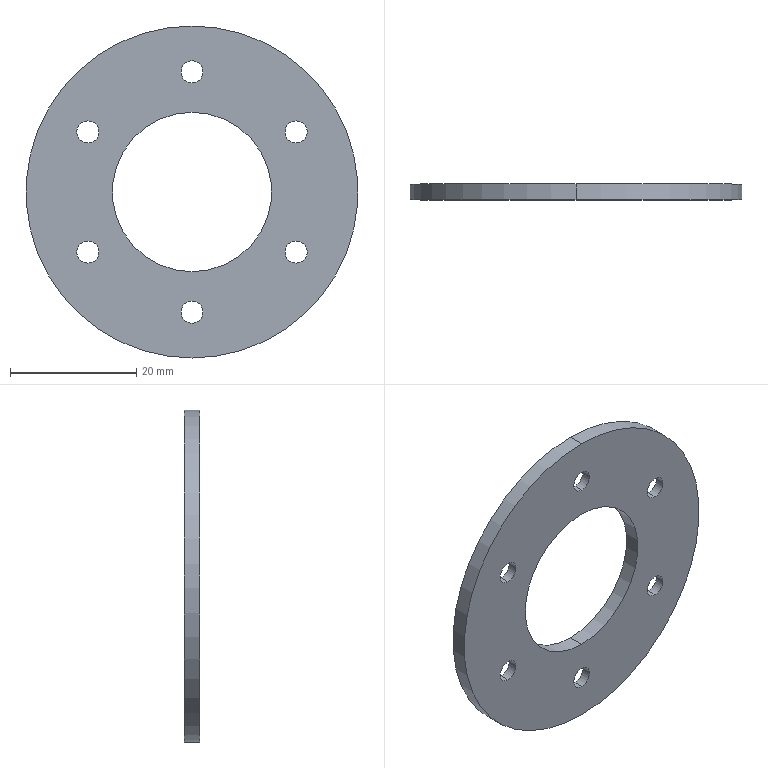Part | SolidWorks | features ICE 4, CirPattern 2, Chamfer 1, Extrusion 1 | 1 solid | 36 faces | box 52.5 x 2.5 x 52.5 mm | volume 3777 mm3 | cylinder 28 | plane 8 | commonest cylinder face diameters 3.5 x12 8 x12 25.2 x2 52.5 x2
STEP:
#1=CARTESIAN_POINT('',(-16.454,1.5,-13.5));
#2=VERTEX_POINT('',#1);
#3=CARTESIAN_POINT('',(-16.454,1.5,-5.5));
#4=VERTEX_POINT('',#3);
#5=CARTESIAN_POINT('',(-16.454,1.5,-9.5));
#6=DIRECTION('',(0.,1.,0.));
#7=DIRECTION('',(0.866,0.,0.5));
#8=AXIS2_PLACEMENT_3D('',#5,#6,#7);
#9=CIRCLE('',#8,4.);
#10=EDGE_CURVE('',#2,#4,#9,.T.);
#11=ORIENTED_EDGE('',*,*,#10,.F.);
#12=CARTESIAN_POINT('',(-16.454,2.5,-13.5));
#13=VERTEX_POINT('',#12);
#14=CARTESIAN_POINT('',(-16.454,1.5,-13.5));
#15=DIRECTION('',(0.,1.,0.));
#16=VECTOR('',#15,1000.);
#17=LINE('',#14,#16);
#18=EDGE_CURVE('',#2,#13,#17,.T.);
#19=ORIENTED_EDGE('',*,*,#18,.T.);
#20=CARTESIAN_POINT('',(-16.454,2.5,-5.5));
#21=VERTEX_POINT('',#20);
#22=CARTESIAN_POINT('',(-16.454,2.5,-9.5));
#23=DIRECTION('',(0.,1.,0.));
#24=DIRECTION('',(0.866,0.,0.5));
#25=AXIS2_PLACEMENT_3D('',#22,#23,#24);
#26=CIRCLE('',#25,4.);
#27=EDGE_CURVE('',#13,#21,#26,.T.);
#28=ORIENTED_EDGE('',*,*,#27,.T.);
#29=CARTESIAN_POINT('',(-16.454,1.5,-5.5));
#30=DIRECTION('',(0.,1.,0.));
#31=VECTOR('',#30,1000.);
#32=LINE('',#29,#31);
#33=EDGE_CURVE('',#4,#21,#32,.T.);
#34=ORIENTED_EDGE('',*,*,#33,.F.);
#35=EDGE_LOOP('',(#11,#19,#28,#34));
#36=FACE_OUTER_BOUND('',#35,.T.);
#37=CARTESIAN_POINT('',(-16.454,1.5,-9.5));
#38=DIRECTION('',(0.,1.,0.));
#39=DIRECTION('',(0.,0.,1.));
#40=AXIS2_PLACEMENT_3D('',#37,#38,#39);
#41=CYLINDRICAL_SURFACE('',#40,4.);
#42=ADVANCED_FACE('',(#36),#41,.F.);
#43=CARTESIAN_POINT('',(-16.454,1.5,5.5));
#44=VERTEX_POINT('',#43);
#45=CARTESIAN_POINT('',(-16.454,1.5,13.5));
#46=VERTEX_POINT('',#45);
#47=CARTESIAN_POINT('',(-16.454,1.5,9.5));
#48=DIRECTION('',(0.,1.,0.));
#49=DIRECTION('',(0.866,0.,-0.5));
#50=AXIS2_PLACEMENT_3D('',#47,#48,#49);
#51=CIRCLE('',#50,4.);
#52=EDGE_CURVE('',#44,#46,#51,.T.);
#53=ORIENTED_EDGE('',*,*,#52,.F.);
#54=CARTESIAN_POINT('',(-16.454,2.5,5.5));
#55=VERTEX_POINT('',#54);
#56=CARTESIAN_POINT('',(-16.454,1.5,5.5));
#57=DIRECTION('',(0.,1.,0.));
#58=VECTOR('',#57,1000.);
#59=LINE('',#56,#58);
#60=EDGE_CURVE('',#44,#55,#59,.T.);
#61=ORIENTED_EDGE('',*,*,#60,.T.);
#62=CARTESIAN_POINT('',(-16.454,2.5,13.5));
#63=VERTEX_POINT('',#62);
#64=CARTESIAN_POINT('',(-16.454,2.5,9.5));
#65=DIRECTION('',(0.,1.,0.));
#66=DIRECTION('',(0.866,0.,-0.5));
#67=AXIS2_PLACEMENT_3D('',#64,#65,#66);
#68=CIRCLE('',#67,4.);
#69=EDGE_CURVE('',#55,#63,#68,.T.);
#70=ORIENTED_EDGE('',*,*,#69,.T.);
#71=CARTESIAN_POINT('',(-16.454,1.5,13.5));
#72=DIRECTION('',(0.,1.,0.));
#73=VECTOR('',#72,1000.);
#74=LINE('',#71,#73);
#75=EDGE_CURVE('',#46,#63,#74,.T.);
#76=ORIENTED_EDGE('',*,*,#75,.F.);
#77=EDGE_LOOP('',(#53,#61,#70,#76));
#78=FACE_OUTER_BOUND('',#77,.T.);
#79=CARTESIAN_POINT('',(-16.454,1.5,9.5));
#80=DIRECTION('',(0.,1.,0.));
#81=DIRECTION('',(0.,0.,1.));
#82=AXIS2_PLACEMENT_3D('',#79,#80,#81);
#83=CYLINDRICAL_SURFACE('',#82,4.);
#84=ADVANCED_FACE('',(#78),#83,.F.);
#85=CARTESIAN_POINT('',(0.,1.5,15.));
#86=VERTEX_POINT('',#85);
#87=CARTESIAN_POINT('',(0.,1.5,23.));
#88=VERTEX_POINT('',#87);
#89=CARTESIAN_POINT('',(0.,1.5,19.));
#90=DIRECTION('',(0.,1.,0.));
#91=DIRECTION('',(0.,0.,-1.));
#92=AXIS2_PLACEMENT_3D('',#89,#90,#91);
#93=CIRCLE('',#92,4.);
#94=EDGE_CURVE('',#86,#88,#93,.T.);
#95=ORIENTED_EDGE('',*,*,#94,.F.);
#96=CARTESIAN_POINT('',(0.,2.5,15.));
#97=VERTEX_POINT('',#96);
#98=CARTESIAN_POINT('',(0.,1.5,15.));
#99=DIRECTION('',(0.,1.,0.));
#100=VECTOR('',#99,1000.);
#101=LINE('',#98,#100);
#102=EDGE_CURVE('',#86,#97,#101,.T.);
#103=ORIENTED_EDGE('',*,*,#102,.T.);
#104=CARTESIAN_POINT('',(0.,2.5,23.));
#105=VERTEX_POINT('',#104);
#106=CARTESIAN_POINT('',(0.,2.5,19.));
#107=DIRECTION('',(0.,1.,0.));
#108=DIRECTION('',(0.,0.,-1.));
#109=AXIS2_PLACEMENT_3D('',#106,#107,#108);
#110=CIRCLE('',#109,4.);
#111=EDGE_CURVE('',#97,#105,#110,.T.);
#112=ORIENTED_EDGE('',*,*,#111,.T.);
#113=CARTESIAN_POINT('',(0.,1.5,23.));
#114=DIRECTION('',(0.,1.,0.));
#115=VECTOR('',#114,1000.);
#116=LINE('',#113,#115);
#117=EDGE_CURVE('',#88,#105,#116,.T.);
#118=ORIENTED_EDGE('',*,*,#117,.F.);
#119=EDGE_LOOP('',(#95,#103,#112,#118));
#120=FACE_OUTER_BOUND('',#119,.T.);
#121=CARTESIAN_POINT('',(0.,1.5,19.));
#122=DIRECTION('',(0.,1.,0.));
#123=DIRECTION('',(0.,0.,1.));
#124=AXIS2_PLACEMENT_3D('',#121,#122,#123);
#125=CYLINDRICAL_SURFACE('',#124,4.);
#126=ADVANCED_FACE('',(#120),#125,.F.);
#127=CARTESIAN_POINT('',(16.454,1.5,5.5));
#128=VERTEX_POINT('',#127);
#129=CARTESIAN_POINT('',(16.454,1.5,13.5));
#130=VERTEX_POINT('',#129);
#131=CARTESIAN_POINT('',(16.454,1.5,9.5));
#132=DIRECTION('',(0.,1.,0.));
#133=DIRECTION('',(-0.866,0.,-0.5));
#134=AXIS2_PLACEMENT_3D('',#131,#132,#133);
#135=CIRCLE('',#134,4.);
#136=EDGE_CURVE('',#128,#130,#135,.T.);
#137=ORIENTED_EDGE('',*,*,#136,.F.);
#138=CARTESIAN_POINT('',(16.454,2.5,5.5));
#139=VERTEX_POINT('',#138);
#140=CARTESIAN_POINT('',(16.454,1.5,5.5));
#141=DIRECTION('',(0.,1.,0.));
#142=VECTOR('',#141,1000.);
#143=LINE('',#140,#142);
#144=EDGE_CURVE('',#128,#139,#143,.T.);
#145=ORIENTED_EDGE('',*,*,#144,.T.);
#146=CARTESIAN_POINT('',(16.454,2.5,13.5));
#147=VERTEX_POINT('',#146);
#148=CARTESIAN_POINT('',(16.454,2.5,9.5));
#149=DIRECTION('',(0.,1.,0.));
#150=DIRECTION('',(-0.866,0.,-0.5));
#151=AXIS2_PLACEMENT_3D('',#148,#149,#150);
#152=CIRCLE('',#151,4.);
#153=EDGE_CURVE('',#139,#147,#152,.T.);
#154=ORIENTED_EDGE('',*,*,#153,.T.);
#155=CARTESIAN_POINT('',(16.454,1.5,13.5));
#156=DIRECTION('',(0.,1.,0.));
#157=VECTOR('',#156,1000.);
#158=LINE('',#155,#157);
#159=EDGE_CURVE('',#130,#147,#158,.T.);
#160=ORIENTED_EDGE('',*,*,#159,.F.);
#161=EDGE_LOOP('',(#137,#145,#154,#160));
#162=FACE_OUTER_BOUND('',#161,.T.);
#163=CARTESIAN_POINT('',(16.454,1.5,9.5));
#164=DIRECTION('',(0.,1.,0.));
#165=DIRECTION('',(0.,0.,1.));
#166=AXIS2_PLACEMENT_3D('',#163,#164,#165);
#167=CYLINDRICAL_SURFACE('',#166,4.);
#168=ADVANCED_FACE('',(#162),#167,.F.);
#169=CARTESIAN_POINT('',(16.454,1.5,-13.5));
#170=VERTEX_POINT('',#169);
#171=CARTESIAN_POINT('',(16.454,1.5,-5.5));
#172=VERTEX_POINT('',#171);
#173=CARTESIAN_POINT('',(16.454,1.5,-9.5));
#174=DIRECTION('',(0.,1.,0.));
#175=DIRECTION('',(-0.866,0.,0.5));
#176=AXIS2_PLACEMENT_3D('',#173,#174,#175);
#177=CIRCLE('',#176,4.);
#178=EDGE_CURVE('',#170,#172,#177,.T.);
#179=ORIENTED_EDGE('',*,*,#178,.F.);
#180=CARTESIAN_POINT('',(16.454,2.5,-13.5));
#181=VERTEX_POINT('',#180);
#182=CARTESIAN_POINT('',(16.454,1.5,-13.5));
#183=DIRECTION('',(0.,1.,0.));
#184=VECTOR('',#183,1000.);
#185=LINE('',#182,#184);
#186=EDGE_CURVE('',#170,#181,#185,.T.);
#187=ORIENTED_EDGE('',*,*,#186,.T.);
#188=CARTESIAN_POINT('',(16.454,2.5,-5.5));
#189=VERTEX_POINT('',#188);
#190=CARTESIAN_POINT('',(16.454,2.5,-9.5));
#191=DIRECTION('',(0.,1.,0.));
#192=DIRECTION('',(-0.866,0.,0.5));
#193=AXIS2_PLACEMENT_3D('',#190,#191,#192);
#194=CIRCLE('',#193,4.);
#195=EDGE_CURVE('',#181,#189,#194,.T.);
#196=ORIENTED_EDGE('',*,*,#195,.T.);
#197=CARTESIAN_POINT('',(16.454,1.5,-5.5));
#198=DIRECTION('',(0.,1.,0.));
#199=VECTOR('',#198,1000.);
#200=LINE('',#197,#199);
#201=EDGE_CURVE('',#172,#189,#200,.T.);
#202=ORIENTED_EDGE('',*,*,#201,.F.);
#203=EDGE_LOOP('',(#179,#187,#196,#202));
#204=FACE_OUTER_BOUND('',#203,.T.);
#205=CARTESIAN_POINT('',(16.454,1.5,-9.5));
#206=DIRECTION('',(0.,1.,0.));
#207=DIRECTION('',(0.,0.,1.));
#208=AXIS2_PLACEMENT_3D('',#205,#206,#207);
#209=CYLINDRICAL_SURFACE('',#208,4.);
#210=ADVANCED_FACE('',(#204),#209,.F.);
#211=CARTESIAN_POINT('',(0.,1.5,-23.));
#212=VERTEX_POINT('',#211);
#213=CARTESIAN_POINT('',(0.,1.5,-15.));
#214=VERTEX_POINT('',#213);
#215=CARTESIAN_POINT('',(0.,1.5,-19.));
#216=DIRECTION('',(0.,1.,0.));
#217=DIRECTION('',(0.,0.,1.));
#218=AXIS2_PLACEMENT_3D('',#215,#216,#217);
#219=CIRCLE('',#218,4.);
#220=EDGE_CURVE('',#212,#214,#219,.T.);
#221=ORIENTED_EDGE('',*,*,#220,.F.);
#222=CARTESIAN_POINT('',(0.,2.5,-23.));
#223=VERTEX_POINT('',#222);
#224=CARTESIAN_POINT('',(0.,1.5,-23.));
#225=DIRECTION('',(0.,1.,0.));
#226=VECTOR('',#225,1000.);
#227=LINE('',#224,#226);
#228=EDGE_CURVE('',#212,#223,#227,.T.);
#229=ORIENTED_EDGE('',*,*,#228,.T.);
#230=CARTESIAN_POINT('',(0.,2.5,-15.));
#231=VERTEX_POINT('',#230);
#232=CARTESIAN_POINT('',(0.,2.5,-19.));
#233=DIRECTION('',(0.,1.,0.));
#234=DIRECTION('',(0.,0.,1.));
#235=AXIS2_PLACEMENT_3D('',#232,#233,#234);
#236=CIRCLE('',#235,4.);
#237=EDGE_CURVE('',#223,#231,#236,.T.);
#238=ORIENTED_EDGE('',*,*,#237,.T.);
#239=CARTESIAN_POINT('',(0.,1.5,-15.));
#240=DIRECTION('',(0.,1.,0.));
#241=VECTOR('',#240,1000.);
#242=LINE('',#239,#241);
#243=EDGE_CURVE('',#214,#231,#242,.T.);
#244=ORIENTED_EDGE('',*,*,#243,.F.);
#245=EDGE_LOOP('',(#221,#229,#238,#244));
#246=FACE_OUTER_BOUND('',#245,.T.);
#247=CARTESIAN_POINT('',(0.,1.5,-19.));
#248=DIRECTION('',(0.,1.,0.));
#249=DIRECTION('',(0.,0.,1.));
#250=AXIS2_PLACEMENT_3D('',#247,#248,#249);
#251=CYLINDRICAL_SURFACE('',#250,4.);
#252=ADVANCED_FACE('',(#246),#251,.F.);
#253=CARTESIAN_POINT('',(0.,2.5,26.25));
#254=VERTEX_POINT('',#253);
#255=CARTESIAN_POINT('',(0.,2.5,-26.25));
#256=VERTEX_POINT('',#255);
#257=CARTESIAN_POINT('',(0.,2.5,0.));
#258=DIRECTION('',(0.,1.,0.));
#259=DIRECTION('',(0.,0.,1.));
#260=AXIS2_PLACEMENT_3D('',#257,#258,#259);
#261=CIRCLE('',#260,26.25);
#262=EDGE_CURVE('',#254,#256,#261,.T.);
#263=ORIENTED_EDGE('',*,*,#262,.F.);
#264=CARTESIAN_POINT('',(0.,0.,26.25));
#265=VERTEX_POINT('',#264);
#266=CARTESIAN_POINT('',(0.,4.,26.25));
#267=DIRECTION('',(0.,-1.,0.));
#268=VECTOR('',#267,1000.);
#269=LINE('',#266,#268);
#270=EDGE_CURVE('',#254,#265,#269,.T.);
#271=ORIENTED_EDGE('',*,*,#270,.T.);
#272=CARTESIAN_POINT('',(0.,0.,-26.25));
#273=VERTEX_POINT('',#272);
#274=CARTESIAN_POINT('',(0.,0.,0.));
#275=DIRECTION('',(0.,1.,0.));
#276=DIRECTION('',(0.,0.,1.));
#277=AXIS2_PLACEMENT_3D('',#274,#275,#276);
#278=CIRCLE('',#277,26.25);
#279=EDGE_CURVE('',#265,#273,#278,.T.);
#280=ORIENTED_EDGE('',*,*,#279,.T.);
#281=CARTESIAN_POINT('',(0.,4.,-26.25));
#282=DIRECTION('',(0.,-1.,0.));
#283=VECTOR('',#282,1000.);
#284=LINE('',#281,#283);
#285=EDGE_CURVE('',#256,#273,#284,.T.);
#286=ORIENTED_EDGE('',*,*,#285,.F.);
#287=EDGE_LOOP('',(#263,#271,#280,#286));
#288=FACE_OUTER_BOUND('',#287,.T.);
#289=CARTESIAN_POINT('',(0.,4.,0.));
#290=DIRECTION('',(0.,-1.,0.));
#291=DIRECTION('',(0.,0.,-1.));
#292=AXIS2_PLACEMENT_3D('',#289,#290,#291);
#293=CYLINDRICAL_SURFACE('',#292,26.25);
#294=ADVANCED_FACE('',(#288),#293,.T.);
#295=CARTESIAN_POINT('',(0.,0.,-20.75));
#296=VERTEX_POINT('',#295);
#297=CARTESIAN_POINT('',(0.,0.,-17.25));
#298=VERTEX_POINT('',#297);
#299=CARTESIAN_POINT('',(0.,0.,-19.));
#300=DIRECTION('',(0.,1.,0.));
#301=DIRECTION('',(0.,0.,1.));
#302=AXIS2_PLACEMENT_3D('',#299,#300,#301);
#303=CIRCLE('',#302,1.75);
#304=EDGE_CURVE('',#296,#298,#303,.T.);
#305=ORIENTED_EDGE('',*,*,#304,.F.);
#306=CARTESIAN_POINT('',(0.,1.5,-20.75));
#307=VERTEX_POINT('',#306);
#308=CARTESIAN_POINT('',(0.,-7.5,-20.75));
#309=DIRECTION('',(0.,1.,0.));
#310=VECTOR('',#309,1000.);
#311=LINE('',#308,#310);
#312=EDGE_CURVE('',#296,#307,#311,.T.);
#313=ORIENTED_EDGE('',*,*,#312,.T.);
#314=CARTESIAN_POINT('',(0.,1.5,-17.25));
#315=VERTEX_POINT('',#314);
#316=CARTESIAN_POINT('',(0.,1.5,-19.));
#317=DIRECTION('',(0.,-1.,0.));
#318=DIRECTION('',(0.,0.,1.));
#319=AXIS2_PLACEMENT_3D('',#316,#317,#318);
#320=CIRCLE('',#319,1.75);
#321=EDGE_CURVE('',#315,#307,#320,.T.);
#322=ORIENTED_EDGE('',*,*,#321,.F.);
#323=CARTESIAN_POINT('',(0.,-7.5,-17.25));
#324=DIRECTION('',(0.,1.,0.));
#325=VECTOR('',#324,1000.);
#326=LINE('',#323,#325);
#327=EDGE_CURVE('',#298,#315,#326,.T.);
#328=ORIENTED_EDGE('',*,*,#327,.F.);
#329=EDGE_LOOP('',(#305,#313,#322,#328));
#330=FACE_OUTER_BOUND('',#329,.T.);
#331=CARTESIAN_POINT('',(0.,-7.5,-19.));
#332=DIRECTION('',(0.,1.,0.));
#333=DIRECTION('',(0.,0.,1.));
#334=AXIS2_PLACEMENT_3D('',#331,#332,#333);
#335=CYLINDRICAL_SURFACE('',#334,1.75);
#336=ADVANCED_FACE('',(#330),#335,.F.);
#337=CARTESIAN_POINT('',(16.454,0.,-11.25));
#338=VERTEX_POINT('',#337);
#339=CARTESIAN_POINT('',(16.454,0.,-7.75));
#340=VERTEX_POINT('',#339);
#341=CARTESIAN_POINT('',(16.454,0.,-9.5));
#342=DIRECTION('',(0.,1.,0.));
#343=DIRECTION('',(0.,0.,1.));
#344=AXIS2_PLACEMENT_3D('',#341,#342,#343);
#345=CIRCLE('',#344,1.75);
#346=EDGE_CURVE('',#338,#340,#345,.T.);
#347=ORIENTED_EDGE('',*,*,#346,.F.);
#348=CARTESIAN_POINT('',(16.454,1.5,-11.25));
#349=VERTEX_POINT('',#348);
#350=CARTESIAN_POINT('',(16.454,-7.5,-11.25));
#351=DIRECTION('',(0.,1.,0.));
#352=VECTOR('',#351,1000.);
#353=LINE('',#350,#352);
#354=EDGE_CURVE('',#338,#349,#353,.T.);
#355=ORIENTED_EDGE('',*,*,#354,.T.);
#356=CARTESIAN_POINT('',(16.454,1.5,-7.75));
#357=VERTEX_POINT('',#356);
#358=CARTESIAN_POINT('',(16.454,1.5,-9.5));
#359=DIRECTION('',(0.,-1.,0.));
#360=DIRECTION('',(0.,0.,1.));
#361=AXIS2_PLACEMENT_3D('',#358,#359,#360);
#362=CIRCLE('',#361,1.75);
#363=EDGE_CURVE('',#357,#349,#362,.T.);
#364=ORIENTED_EDGE('',*,*,#363,.F.);
#365=CARTESIAN_POINT('',(16.454,-7.5,-7.75));
#366=DIRECTION('',(0.,1.,0.));
#367=VECTOR('',#366,1000.);
#368=LINE('',#365,#367);
#369=EDGE_CURVE('',#340,#357,#368,.T.);
#370=ORIENTED_EDGE('',*,*,#369,.F.);
#371=EDGE_LOOP('',(#347,#355,#364,#370));
#372=FACE_OUTER_BOUND('',#371,.T.);
#373=CARTESIAN_POINT('',(16.454,-7.5,-9.5));
#374=DIRECTION('',(0.,1.,0.));
#375=DIRECTION('',(0.,0.,1.));
#376=AXIS2_PLACEMENT_3D('',#373,#374,#375);
#377=CYLINDRICAL_SURFACE('',#376,1.75);
#378=ADVANCED_FACE('',(#372),#377,.F.);
#379=CARTESIAN_POINT('',(16.454,0.,7.75));
#380=VERTEX_POINT('',#379);
#381=CARTESIAN_POINT('',(16.454,0.,11.25));
#382=VERTEX_POINT('',#381);
#383=CARTESIAN_POINT('',(16.454,0.,9.5));
#384=DIRECTION('',(0.,1.,0.));
#385=DIRECTION('',(0.,0.,1.));
#386=AXIS2_PLACEMENT_3D('',#383,#384,#385);
#387=CIRCLE('',#386,1.75);
#388=EDGE_CURVE('',#380,#382,#387,.T.);
#389=ORIENTED_EDGE('',*,*,#388,.F.);
#390=CARTESIAN_POINT('',(16.454,1.5,7.75));
#391=VERTEX_POINT('',#390);
#392=CARTESIAN_POINT('',(16.454,-7.5,7.75));
#393=DIRECTION('',(0.,1.,0.));
#394=VECTOR('',#393,1000.);
#395=LINE('',#392,#394);
#396=EDGE_CURVE('',#380,#391,#395,.T.);
#397=ORIENTED_EDGE('',*,*,#396,.T.);
#398=CARTESIAN_POINT('',(16.454,1.5,11.25));
#399=VERTEX_POINT('',#398);
#400=CARTESIAN_POINT('',(16.454,1.5,9.5));
#401=DIRECTION('',(0.,-1.,0.));
#402=DIRECTION('',(0.,0.,1.));
#403=AXIS2_PLACEMENT_3D('',#400,#401,#402);
#404=CIRCLE('',#403,1.75);
#405=EDGE_CURVE('',#399,#391,#404,.T.);
#406=ORIENTED_EDGE('',*,*,#405,.F.);
#407=CARTESIAN_POINT('',(16.454,-7.5,11.25));
#408=DIRECTION('',(0.,1.,0.));
#409=VECTOR('',#408,1000.);
#410=LINE('',#407,#409);
#411=EDGE_CURVE('',#382,#399,#410,.T.);
#412=ORIENTED_EDGE('',*,*,#411,.F.);
#413=EDGE_LOOP('',(#389,#397,#406,#412));
#414=FACE_OUTER_BOUND('',#413,.T.);
#415=CARTESIAN_POINT('',(16.454,-7.5,9.5));
#416=DIRECTION('',(0.,1.,0.));
#417=DIRECTION('',(0.,0.,1.));
#418=AXIS2_PLACEMENT_3D('',#415,#416,#417);
#419=CYLINDRICAL_SURFACE('',#418,1.75);
#420=ADVANCED_FACE('',(#414),#419,.F.);
#421=CARTESIAN_POINT('',(0.,0.,17.25));
#422=VERTEX_POINT('',#421);
#423=CARTESIAN_POINT('',(0.,0.,20.75));
#424=VERTEX_POINT('',#423);
#425=CARTESIAN_POINT('',(0.,0.,19.));
#426=DIRECTION('',(0.,1.,0.));
#427=DIRECTION('',(0.,0.,1.));
#428=AXIS2_PLACEMENT_3D('',#425,#426,#427);
#429=CIRCLE('',#428,1.75);
#430=EDGE_CURVE('',#422,#424,#429,.T.);
#431=ORIENTED_EDGE('',*,*,#430,.F.);
#432=CARTESIAN_POINT('',(0.,1.5,17.25));
#433=VERTEX_POINT('',#432);
#434=CARTESIAN_POINT('',(0.,-7.5,17.25));
#435=DIRECTION('',(0.,1.,0.));
#436=VECTOR('',#435,1000.);
#437=LINE('',#434,#436);
#438=EDGE_CURVE('',#422,#433,#437,.T.);
#439=ORIENTED_EDGE('',*,*,#438,.T.);
#440=CARTESIAN_POINT('',(0.,1.5,20.75));
#441=VERTEX_POINT('',#440);
#442=CARTESIAN_POINT('',(0.,1.5,19.));
#443=DIRECTION('',(0.,-1.,0.));
#444=DIRECTION('',(0.,0.,1.));
#445=AXIS2_PLACEMENT_3D('',#442,#443,#444);
#446=CIRCLE('',#445,1.75);
#447=EDGE_CURVE('',#441,#433,#446,.T.);
#448=ORIENTED_EDGE('',*,*,#447,.F.);
#449=CARTESIAN_POINT('',(0.,-7.5,20.75));
#450=DIRECTION('',(0.,1.,0.));
#451=VECTOR('',#450,1000.);
#452=LINE('',#449,#451);
#453=EDGE_CURVE('',#424,#441,#452,.T.);
#454=ORIENTED_EDGE('',*,*,#453,.F.);
#455=EDGE_LOOP('',(#431,#439,#448,#454));
#456=FACE_OUTER_BOUND('',#455,.T.);
#457=CARTESIAN_POINT('',(0.,-7.5,19.));
#458=DIRECTION('',(0.,1.,0.));
#459=DIRECTION('',(0.,0.,1.));
#460=AXIS2_PLACEMENT_3D('',#457,#458,#459);
#461=CYLINDRICAL_SURFACE('',#460,1.75);
#462=ADVANCED_FACE('',(#456),#461,.F.);
#463=CARTESIAN_POINT('',(-16.454,0.,7.75));
#464=VERTEX_POINT('',#463);
#465=CARTESIAN_POINT('',(-16.454,0.,11.25));
#466=VERTEX_POINT('',#465);
#467=CARTESIAN_POINT('',(-16.454,0.,9.5));
#468=DIRECTION('',(0.,1.,0.));
#469=DIRECTION('',(0.,0.,1.));
#470=AXIS2_PLACEMENT_3D('',#467,#468,#469);
#471=CIRCLE('',#470,1.75);
#472=EDGE_CURVE('',#464,#466,#471,.T.);
#473=ORIENTED_EDGE('',*,*,#472,.F.);
#474=CARTESIAN_POINT('',(-16.454,1.5,7.75));
#475=VERTEX_POINT('',#474);
#476=CARTESIAN_POINT('',(-16.454,-7.5,7.75));
#477=DIRECTION('',(0.,1.,0.));
#478=VECTOR('',#477,1000.);
#479=LINE('',#476,#478);
#480=EDGE_CURVE('',#464,#475,#479,.T.);
#481=ORIENTED_EDGE('',*,*,#480,.T.);
#482=CARTESIAN_POINT('',(-16.454,1.5,11.25));
#483=VERTEX_POINT('',#482);
#484=CARTESIAN_POINT('',(-16.454,1.5,9.5));
#485=DIRECTION('',(0.,-1.,0.));
#486=DIRECTION('',(0.,0.,1.));
#487=AXIS2_PLACEMENT_3D('',#484,#485,#486);
#488=CIRCLE('',#487,1.75);
#489=EDGE_CURVE('',#483,#475,#488,.T.);
#490=ORIENTED_EDGE('',*,*,#489,.F.);
#491=CARTESIAN_POINT('',(-16.454,-7.5,11.25));
#492=DIRECTION('',(0.,1.,0.));
#493=VECTOR('',#492,1000.);
#494=LINE('',#491,#493);
#495=EDGE_CURVE('',#466,#483,#494,.T.);
#496=ORIENTED_EDGE('',*,*,#495,.F.);
#497=EDGE_LOOP('',(#473,#481,#490,#496));
#498=FACE_OUTER_BOUND('',#497,.T.);
#499=CARTESIAN_POINT('',(-16.454,-7.5,9.5));
#500=DIRECTION('',(0.,1.,0.));
#501=DIRECTION('',(0.,0.,1.));
#502=AXIS2_PLACEMENT_3D('',#499,#500,#501);
#503=CYLINDRICAL_SURFACE('',#502,1.75);
#504=ADVANCED_FACE('',(#498),#503,.F.);
#505=CARTESIAN_POINT('',(-16.454,0.,-11.25));
#506=VERTEX_POINT('',#505);
#507=CARTESIAN_POINT('',(-16.454,0.,-7.75));
#508=VERTEX_POINT('',#507);
#509=CARTESIAN_POINT('',(-16.454,0.,-9.5));
#510=DIRECTION('',(0.,1.,0.));
#511=DIRECTION('',(0.,0.,1.));
#512=AXIS2_PLACEMENT_3D('',#509,#510,#511);
#513=CIRCLE('',#512,1.75);
#514=EDGE_CURVE('',#506,#508,#513,.T.);
#515=ORIENTED_EDGE('',*,*,#514,.F.);
#516=CARTESIAN_POINT('',(-16.454,1.5,-11.25));
#517=VERTEX_POINT('',#516);
#518=CARTESIAN_POINT('',(-16.454,-7.5,-11.25));
#519=DIRECTION('',(0.,1.,0.));
#520=VECTOR('',#519,1000.);
#521=LINE('',#518,#520);
#522=EDGE_CURVE('',#506,#517,#521,.T.);
#523=ORIENTED_EDGE('',*,*,#522,.T.);
#524=CARTESIAN_POINT('',(-16.454,1.5,-7.75));
#525=VERTEX_POINT('',#524);
#526=CARTESIAN_POINT('',(-16.454,1.5,-9.5));
#527=DIRECTION('',(0.,-1.,0.));
#528=DIRECTION('',(0.,0.,1.));
#529=AXIS2_PLACEMENT_3D('',#526,#527,#528);
#530=CIRCLE('',#529,1.75);
#531=EDGE_CURVE('',#525,#517,#530,.T.);
#532=ORIENTED_EDGE('',*,*,#531,.F.);
#533=CARTESIAN_POINT('',(-16.454,-7.5,-7.75));
#534=DIRECTION('',(0.,1.,0.));
#535=VECTOR('',#534,1000.);
#536=LINE('',#533,#535);
#537=EDGE_CURVE('',#508,#525,#536,.T.);
#538=ORIENTED_EDGE('',*,*,#537,.F.);
#539=EDGE_LOOP('',(#515,#523,#532,#538));
#540=FACE_OUTER_BOUND('',#539,.T.);
#541=CARTESIAN_POINT('',(-16.454,-7.5,-9.5));
#542=DIRECTION('',(0.,1.,0.));
#543=DIRECTION('',(0.,0.,1.));
#544=AXIS2_PLACEMENT_3D('',#541,#542,#543);
#545=CYLINDRICAL_SURFACE('',#544,1.75);
#546=ADVANCED_FACE('',(#540),#545,.F.);
#547=CARTESIAN_POINT('',(0.,2.5,-12.6));
#548=VERTEX_POINT('',#547);
#549=CARTESIAN_POINT('',(0.,2.5,12.6));
#550=VERTEX_POINT('',#549);
#551=CARTESIAN_POINT('',(0.,2.5,0.));
#552=DIRECTION('',(0.,1.,0.));
#553=DIRECTION('',(0.,0.,1.));
#554=AXIS2_PLACEMENT_3D('',#551,#552,#553);
#555=CIRCLE('',#554,12.6);
#556=EDGE_CURVE('',#548,#550,#555,.T.);
#557=ORIENTED_EDGE('',*,*,#556,.T.);
#558=CARTESIAN_POINT('',(0.,0.,12.6));
#559=VERTEX_POINT('',#558);
#560=CARTESIAN_POINT('',(0.,4.,12.6));
#561=DIRECTION('',(0.,-1.,0.));
#562=VECTOR('',#561,1000.);
#563=LINE('',#560,#562);
#564=EDGE_CURVE('',#550,#559,#563,.T.);
#565=ORIENTED_EDGE('',*,*,#564,.T.);
#566=CARTESIAN_POINT('',(0.,0.,-12.6));
#567=VERTEX_POINT('',#566);
#568=CARTESIAN_POINT('',(0.,0.,0.));
#569=DIRECTION('',(0.,1.,0.));
#570=DIRECTION('',(0.,0.,1.));
#571=AXIS2_PLACEMENT_3D('',#568,#569,#570);
#572=CIRCLE('',#571,12.6);
#573=EDGE_CURVE('',#567,#559,#572,.T.);
#574=ORIENTED_EDGE('',*,*,#573,.F.);
#575=CARTESIAN_POINT('',(0.,4.,-12.6));
#576=DIRECTION('',(0.,-1.,0.));
#577=VECTOR('',#576,1000.);
#578=LINE('',#575,#577);
#579=EDGE_CURVE('',#548,#567,#578,.T.);
#580=ORIENTED_EDGE('',*,*,#579,.F.);
#581=EDGE_LOOP('',(#557,#565,#574,#580));
#582=FACE_OUTER_BOUND('',#581,.T.);
#583=CARTESIAN_POINT('',(0.,4.,0.));
#584=DIRECTION('',(0.,-1.,0.));
#585=DIRECTION('',(0.,0.,-1.));
#586=AXIS2_PLACEMENT_3D('',#583,#584,#585);
#587=CYLINDRICAL_SURFACE('',#586,12.6);
#588=ADVANCED_FACE('',(#582),#587,.F.);
#589=ORIENTED_EDGE('',*,*,#564,.F.);
#590=CARTESIAN_POINT('',(0.,2.5,0.));
#591=DIRECTION('',(0.,1.,0.));
#592=DIRECTION('',(0.,0.,1.));
#593=AXIS2_PLACEMENT_3D('',#590,#591,#592);
#594=CIRCLE('',#593,12.6);
#595=EDGE_CURVE('',#550,#548,#594,.T.);
#596=ORIENTED_EDGE('',*,*,#595,.T.);
#597=ORIENTED_EDGE('',*,*,#579,.T.);
#598=CARTESIAN_POINT('',(0.,0.,0.));
#599=DIRECTION('',(0.,1.,0.));
#600=DIRECTION('',(0.,0.,1.));
#601=AXIS2_PLACEMENT_3D('',#598,#599,#600);
#602=CIRCLE('',#601,12.6);
#603=EDGE_CURVE('',#559,#567,#602,.T.);
#604=ORIENTED_EDGE('',*,*,#603,.F.);
#605=EDGE_LOOP('',(#589,#596,#597,#604));
#606=FACE_OUTER_BOUND('',#605,.T.);
#607=CARTESIAN_POINT('',(0.,4.,0.));
#608=DIRECTION('',(0.,-1.,0.));
#609=DIRECTION('',(0.,0.,-1.));
#610=AXIS2_PLACEMENT_3D('',#607,#608,#609);
#611=CYLINDRICAL_SURFACE('',#610,12.6);
#612=ADVANCED_FACE('',(#606),#611,.F.);
#613=ORIENTED_EDGE('',*,*,#522,.F.);
#614=CARTESIAN_POINT('',(-16.454,0.,-9.5));
#615=DIRECTION('',(0.,1.,0.));
#616=DIRECTION('',(0.,0.,1.));
#617=AXIS2_PLACEMENT_3D('',#614,#615,#616);
#618=CIRCLE('',#617,1.75);
#619=EDGE_CURVE('',#508,#506,#618,.T.);
#620=ORIENTED_EDGE('',*,*,#619,.F.);
#621=ORIENTED_EDGE('',*,*,#537,.T.);
#622=CARTESIAN_POINT('',(-16.454,1.5,-9.5));
#623=DIRECTION('',(0.,-1.,0.));
#624=DIRECTION('',(0.,0.,1.));
#625=AXIS2_PLACEMENT_3D('',#622,#623,#624);
#626=CIRCLE('',#625,1.75);
#627=EDGE_CURVE('',#517,#525,#626,.T.);
#628=ORIENTED_EDGE('',*,*,#627,.F.);
#629=EDGE_LOOP('',(#613,#620,#621,#628));
#630=FACE_OUTER_BOUND('',#629,.T.);
#631=CARTESIAN_POINT('',(-16.454,-7.5,-9.5));
#632=DIRECTION('',(0.,1.,0.));
#633=DIRECTION('',(0.,0.,1.));
#634=AXIS2_PLACEMENT_3D('',#631,#632,#633);
#635=CYLINDRICAL_SURFACE('',#634,1.75);
#636=ADVANCED_FACE('',(#630),#635,.F.);
#637=ORIENTED_EDGE('',*,*,#480,.F.);
#638=CARTESIAN_POINT('',(-16.454,0.,9.5));
#639=DIRECTION('',(0.,1.,0.));
#640=DIRECTION('',(0.,0.,1.));
#641=AXIS2_PLACEMENT_3D('',#638,#639,#640);
#642=CIRCLE('',#641,1.75);
#643=EDGE_CURVE('',#466,#464,#642,.T.);
#644=ORIENTED_EDGE('',*,*,#643,.F.);
#645=ORIENTED_EDGE('',*,*,#495,.T.);
#646=CARTESIAN_POINT('',(-16.454,1.5,9.5));
#647=DIRECTION('',(0.,-1.,0.));
#648=DIRECTION('',(0.,0.,1.));
#649=AXIS2_PLACEMENT_3D('',#646,#647,#648);
#650=CIRCLE('',#649,1.75);
#651=EDGE_CURVE('',#475,#483,#650,.T.);
#652=ORIENTED_EDGE('',*,*,#651,.F.);
#653=EDGE_LOOP('',(#637,#644,#645,#652));
#654=FACE_OUTER_BOUND('',#653,.T.);
#655=CARTESIAN_POINT('',(-16.454,-7.5,9.5));
#656=DIRECTION('',(0.,1.,0.));
#657=DIRECTION('',(0.,0.,1.));
#658=AXIS2_PLACEMENT_3D('',#655,#656,#657);
#659=CYLINDRICAL_SURFACE('',#658,1.75);
#660=ADVANCED_FACE('',(#654),#659,.F.);
#661=ORIENTED_EDGE('',*,*,#438,.F.);
#662=CARTESIAN_POINT('',(0.,0.,19.));
#663=DIRECTION('',(0.,1.,0.));
#664=DIRECTION('',(0.,0.,1.));
#665=AXIS2_PLACEMENT_3D('',#662,#663,#664);
#666=CIRCLE('',#665,1.75);
#667=EDGE_CURVE('',#424,#422,#666,.T.);
#668=ORIENTED_EDGE('',*,*,#667,.F.);
#669=ORIENTED_EDGE('',*,*,#453,.T.);
#670=CARTESIAN_POINT('',(0.,1.5,19.));
#671=DIRECTION('',(0.,-1.,0.));
#672=DIRECTION('',(0.,0.,1.));
#673=AXIS2_PLACEMENT_3D('',#670,#671,#672);
#674=CIRCLE('',#673,1.75);
#675=EDGE_CURVE('',#433,#441,#674,.T.);
#676=ORIENTED_EDGE('',*,*,#675,.F.);
#677=EDGE_LOOP('',(#661,#668,#669,#676));
#678=FACE_OUTER_BOUND('',#677,.T.);
#679=CARTESIAN_POINT('',(0.,-7.5,19.));
#680=DIRECTION('',(0.,1.,0.));
#681=DIRECTION('',(0.,0.,1.));
#682=AXIS2_PLACEMENT_3D('',#679,#680,#681);
#683=CYLINDRICAL_SURFACE('',#682,1.75);
#684=ADVANCED_FACE('',(#678),#683,.F.);
#685=ORIENTED_EDGE('',*,*,#396,.F.);
#686=CARTESIAN_POINT('',(16.454,0.,9.5));
#687=DIRECTION('',(0.,1.,0.));
#688=DIRECTION('',(0.,0.,1.));
#689=AXIS2_PLACEMENT_3D('',#686,#687,#688);
#690=CIRCLE('',#689,1.75);
#691=EDGE_CURVE('',#382,#380,#690,.T.);
#692=ORIENTED_EDGE('',*,*,#691,.F.);
#693=ORIENTED_EDGE('',*,*,#411,.T.);
#694=CARTESIAN_POINT('',(16.454,1.5,9.5));
#695=DIRECTION('',(0.,-1.,0.));
#696=DIRECTION('',(0.,0.,1.));
#697=AXIS2_PLACEMENT_3D('',#694,#695,#696);
#698=CIRCLE('',#697,1.75);
#699=EDGE_CURVE('',#391,#399,#698,.T.);
#700=ORIENTED_EDGE('',*,*,#699,.F.);
#701=EDGE_LOOP('',(#685,#692,#693,#700));
#702=FACE_OUTER_BOUND('',#701,.T.);
#703=CARTESIAN_POINT('',(16.454,-7.5,9.5));
#704=DIRECTION('',(0.,1.,0.));
#705=DIRECTION('',(0.,0.,1.));
#706=AXIS2_PLACEMENT_3D('',#703,#704,#705);
#707=CYLINDRICAL_SURFACE('',#706,1.75);
#708=ADVANCED_FACE('',(#702),#707,.F.);
#709=ORIENTED_EDGE('',*,*,#354,.F.);
#710=CARTESIAN_POINT('',(16.454,0.,-9.5));
#711=DIRECTION('',(0.,1.,0.));
#712=DIRECTION('',(0.,0.,1.));
#713=AXIS2_PLACEMENT_3D('',#710,#711,#712);
#714=CIRCLE('',#713,1.75);
#715=EDGE_CURVE('',#340,#338,#714,.T.);
#716=ORIENTED_EDGE('',*,*,#715,.F.);
#717=ORIENTED_EDGE('',*,*,#369,.T.);
#718=CARTESIAN_POINT('',(16.454,1.5,-9.5));
#719=DIRECTION('',(0.,-1.,0.));
#720=DIRECTION('',(0.,0.,1.));
#721=AXIS2_PLACEMENT_3D('',#718,#719,#720);
#722=CIRCLE('',#721,1.75);
#723=EDGE_CURVE('',#349,#357,#722,.T.);
#724=ORIENTED_EDGE('',*,*,#723,.F.);
#725=EDGE_LOOP('',(#709,#716,#717,#724));
#726=FACE_OUTER_BOUND('',#725,.T.);
#727=CARTESIAN_POINT('',(16.454,-7.5,-9.5));
#728=DIRECTION('',(0.,1.,0.));
#729=DIRECTION('',(0.,0.,1.));
#730=AXIS2_PLACEMENT_3D('',#727,#728,#729);
#731=CYLINDRICAL_SURFACE('',#730,1.75);
#732=ADVANCED_FACE('',(#726),#731,.F.);
#733=ORIENTED_EDGE('',*,*,#312,.F.);
#734=CARTESIAN_POINT('',(0.,0.,-19.));
#735=DIRECTION('',(0.,1.,0.));
#736=DIRECTION('',(0.,0.,1.));
#737=AXIS2_PLACEMENT_3D('',#734,#735,#736);
#738=CIRCLE('',#737,1.75);
#739=EDGE_CURVE('',#298,#296,#738,.T.);
#740=ORIENTED_EDGE('',*,*,#739,.F.);
#741=ORIENTED_EDGE('',*,*,#327,.T.);
#742=CARTESIAN_POINT('',(0.,1.5,-19.));
#743=DIRECTION('',(0.,-1.,0.));
#744=DIRECTION('',(0.,0.,1.));
#745=AXIS2_PLACEMENT_3D('',#742,#743,#744);
#746=CIRCLE('',#745,1.75);
#747=EDGE_CURVE('',#307,#315,#746,.T.);
#748=ORIENTED_EDGE('',*,*,#747,.F.);
#749=EDGE_LOOP('',(#733,#740,#741,#748));
#750=FACE_OUTER_BOUND('',#749,.T.);
#751=CARTESIAN_POINT('',(0.,-7.5,-19.));
#752=DIRECTION('',(0.,1.,0.));
#753=DIRECTION('',(0.,0.,1.));
#754=AXIS2_PLACEMENT_3D('',#751,#752,#753);
#755=CYLINDRICAL_SURFACE('',#754,1.75);
#756=ADVANCED_FACE('',(#750),#755,.F.);
#757=ORIENTED_EDGE('',*,*,#270,.F.);
#758=CARTESIAN_POINT('',(0.,2.5,0.));
#759=DIRECTION('',(0.,1.,0.));
#760=DIRECTION('',(0.,0.,1.));
#761=AXIS2_PLACEMENT_3D('',#758,#759,#760);
#762=CIRCLE('',#761,26.25);
#763=EDGE_CURVE('',#256,#254,#762,.T.);
#764=ORIENTED_EDGE('',*,*,#763,.F.);
#765=ORIENTED_EDGE('',*,*,#285,.T.);
#766=CARTESIAN_POINT('',(0.,0.,0.));
#767=DIRECTION('',(0.,1.,0.));
#768=DIRECTION('',(0.,0.,1.));
#769=AXIS2_PLACEMENT_3D('',#766,#767,#768);
#770=CIRCLE('',#769,26.25);
#771=EDGE_CURVE('',#273,#265,#770,.T.);
#772=ORIENTED_EDGE('',*,*,#771,.T.);
#773=EDGE_LOOP('',(#757,#764,#765,#772));
#774=FACE_OUTER_BOUND('',#773,.T.);
#775=CARTESIAN_POINT('',(0.,4.,0.));
#776=DIRECTION('',(0.,-1.,0.));
#777=DIRECTION('',(0.,0.,-1.));
#778=AXIS2_PLACEMENT_3D('',#775,#776,#777);
#779=CYLINDRICAL_SURFACE('',#778,26.25);
#780=ADVANCED_FACE('',(#774),#779,.T.);
#781=ORIENTED_EDGE('',*,*,#619,.T.);
#782=ORIENTED_EDGE('',*,*,#514,.T.);
#783=EDGE_LOOP('',(#781,#782));
#784=FACE_BOUND('',#783,.T.);
#785=ORIENTED_EDGE('',*,*,#643,.T.);
#786=ORIENTED_EDGE('',*,*,#472,.T.);
#787=EDGE_LOOP('',(#785,#786));
#788=FACE_BOUND('',#787,.T.);
#789=ORIENTED_EDGE('',*,*,#667,.T.);
#790=ORIENTED_EDGE('',*,*,#430,.T.);
#791=EDGE_LOOP('',(#789,#790));
#792=FACE_BOUND('',#791,.T.);
#793=ORIENTED_EDGE('',*,*,#691,.T.);
#794=ORIENTED_EDGE('',*,*,#388,.T.);
#795=EDGE_LOOP('',(#793,#794));
#796=FACE_BOUND('',#795,.T.);
#797=ORIENTED_EDGE('',*,*,#715,.T.);
#798=ORIENTED_EDGE('',*,*,#346,.T.);
#799=EDGE_LOOP('',(#797,#798));
#800=FACE_BOUND('',#799,.T.);
#801=ORIENTED_EDGE('',*,*,#739,.T.);
#802=ORIENTED_EDGE('',*,*,#304,.T.);
#803=EDGE_LOOP('',(#801,#802));
#804=FACE_BOUND('',#803,.T.);
#805=ORIENTED_EDGE('',*,*,#771,.F.);
#806=ORIENTED_EDGE('',*,*,#279,.F.);
#807=EDGE_LOOP('',(#805,#806));
#808=FACE_OUTER_BOUND('',#807,.T.);
#809=ORIENTED_EDGE('',*,*,#573,.T.);
#810=ORIENTED_EDGE('',*,*,#603,.T.);
#811=EDGE_LOOP('',(#809,#810));
#812=FACE_BOUND('',#811,.T.);
#813=CARTESIAN_POINT('',(0.,0.,0.));
#814=DIRECTION('',(0.,1.,0.));
#815=DIRECTION('',(0.,0.,1.));
#816=AXIS2_PLACEMENT_3D('',#813,#814,#815);
#817=PLANE('',#816);
#818=ADVANCED_FACE('',(#784,#788,#792,#796,#800,#804,#808,#812),#817,.F.);
#819=CARTESIAN_POINT('',(-16.454,2.5,-9.5));
#820=DIRECTION('',(0.,1.,0.));
#821=DIRECTION('',(0.866,0.,0.5));
#822=AXIS2_PLACEMENT_3D('',#819,#820,#821);
#823=CIRCLE('',#822,4.);
#824=EDGE_CURVE('',#21,#13,#823,.T.);
#825=ORIENTED_EDGE('',*,*,#824,.F.);
#826=ORIENTED_EDGE('',*,*,#27,.F.);
#827=EDGE_LOOP('',(#825,#826));
#828=FACE_BOUND('',#827,.T.);
#829=CARTESIAN_POINT('',(-16.454,2.5,9.5));
#830=DIRECTION('',(0.,1.,0.));
#831=DIRECTION('',(0.866,0.,-0.5));
#832=AXIS2_PLACEMENT_3D('',#829,#830,#831);
#833=CIRCLE('',#832,4.);
#834=EDGE_CURVE('',#63,#55,#833,.T.);
#835=ORIENTED_EDGE('',*,*,#834,.F.);
#836=ORIENTED_EDGE('',*,*,#69,.F.);
#837=EDGE_LOOP('',(#835,#836));
#838=FACE_BOUND('',#837,.T.);
#839=CARTESIAN_POINT('',(0.,2.5,19.));
#840=DIRECTION('',(0.,1.,0.));
#841=DIRECTION('',(0.,0.,-1.));
#842=AXIS2_PLACEMENT_3D('',#839,#840,#841);
#843=CIRCLE('',#842,4.);
#844=EDGE_CURVE('',#105,#97,#843,.T.);
#845=ORIENTED_EDGE('',*,*,#844,.F.);
#846=ORIENTED_EDGE('',*,*,#111,.F.);
#847=EDGE_LOOP('',(#845,#846));
#848=FACE_BOUND('',#847,.T.);
#849=CARTESIAN_POINT('',(16.454,2.5,9.5));
#850=DIRECTION('',(0.,1.,0.));
#851=DIRECTION('',(-0.866,0.,-0.5));
#852=AXIS2_PLACEMENT_3D('',#849,#850,#851);
#853=CIRCLE('',#852,4.);
#854=EDGE_CURVE('',#147,#139,#853,.T.);
#855=ORIENTED_EDGE('',*,*,#854,.F.);
#856=ORIENTED_EDGE('',*,*,#153,.F.);
#857=EDGE_LOOP('',(#855,#856));
#858=FACE_BOUND('',#857,.T.);
#859=CARTESIAN_POINT('',(16.454,2.5,-9.5));
#860=DIRECTION('',(0.,1.,0.));
#861=DIRECTION('',(-0.866,0.,0.5));
#862=AXIS2_PLACEMENT_3D('',#859,#860,#861);
#863=CIRCLE('',#862,4.);
#864=EDGE_CURVE('',#189,#181,#863,.T.);
#865=ORIENTED_EDGE('',*,*,#864,.F.);
#866=ORIENTED_EDGE('',*,*,#195,.F.);
#867=EDGE_LOOP('',(#865,#866));
#868=FACE_BOUND('',#867,.T.);
#869=CARTESIAN_POINT('',(0.,2.5,-19.));
#870=DIRECTION('',(0.,1.,0.));
#871=DIRECTION('',(0.,0.,1.));
#872=AXIS2_PLACEMENT_3D('',#869,#870,#871);
#873=CIRCLE('',#872,4.);
#874=EDGE_CURVE('',#231,#223,#873,.T.);
#875=ORIENTED_EDGE('',*,*,#874,.F.);
#876=ORIENTED_EDGE('',*,*,#237,.F.);
#877=EDGE_LOOP('',(#875,#876));
#878=FACE_BOUND('',#877,.T.);
#879=ORIENTED_EDGE('',*,*,#763,.T.);
#880=ORIENTED_EDGE('',*,*,#262,.T.);
#881=EDGE_LOOP('',(#879,#880));
#882=FACE_OUTER_BOUND('',#881,.T.);
#883=ORIENTED_EDGE('',*,*,#556,.F.);
#884=ORIENTED_EDGE('',*,*,#595,.F.);
#885=EDGE_LOOP('',(#883,#884));
#886=FACE_BOUND('',#885,.T.);
#887=CARTESIAN_POINT('',(0.,2.5,0.));
#888=DIRECTION('',(0.,1.,0.));
#889=DIRECTION('',(0.,0.,1.));
#890=AXIS2_PLACEMENT_3D('',#887,#888,#889);
#891=PLANE('',#890);
#892=ADVANCED_FACE('',(#828,#838,#848,#858,#868,#878,#882,#886),#891,.T.);
#893=CARTESIAN_POINT('',(0.,1.5,-19.));
#894=DIRECTION('',(0.,1.,0.));
#895=DIRECTION('',(0.,0.,1.));
#896=AXIS2_PLACEMENT_3D('',#893,#894,#895);
#897=CIRCLE('',#896,4.);
#898=EDGE_CURVE('',#214,#212,#897,.T.);
#899=ORIENTED_EDGE('',*,*,#898,.T.);
#900=ORIENTED_EDGE('',*,*,#220,.T.);
#901=EDGE_LOOP('',(#899,#900));
#902=FACE_OUTER_BOUND('',#901,.T.);
#903=ORIENTED_EDGE('',*,*,#321,.T.);
#904=ORIENTED_EDGE('',*,*,#747,.T.);
#905=EDGE_LOOP('',(#903,#904));
#906=FACE_BOUND('',#905,.T.);
#907=CARTESIAN_POINT('',(0.,1.5,-19.));
#908=DIRECTION('',(0.,1.,0.));
#909=DIRECTION('',(0.,0.,1.));
#910=AXIS2_PLACEMENT_3D('',#907,#908,#909);
#911=PLANE('',#910);
#912=ADVANCED_FACE('',(#902,#906),#911,.T.);
#913=ORIENTED_EDGE('',*,*,#228,.F.);
#914=ORIENTED_EDGE('',*,*,#898,.F.);
#915=ORIENTED_EDGE('',*,*,#243,.T.);
#916=ORIENTED_EDGE('',*,*,#874,.T.);
#917=EDGE_LOOP('',(#913,#914,#915,#916));
#918=FACE_OUTER_BOUND('',#917,.T.);
#919=CARTESIAN_POINT('',(0.,1.5,-19.));
#920=DIRECTION('',(0.,1.,0.));
#921=DIRECTION('',(0.,0.,1.));
#922=AXIS2_PLACEMENT_3D('',#919,#920,#921);
#923=CYLINDRICAL_SURFACE('',#922,4.);
#924=ADVANCED_FACE('',(#918),#923,.F.);
#925=CARTESIAN_POINT('',(16.454,1.5,-9.5));
#926=DIRECTION('',(0.,1.,0.));
#927=DIRECTION('',(-0.866,0.,0.5));
#928=AXIS2_PLACEMENT_3D('',#925,#926,#927);
#929=CIRCLE('',#928,4.);
#930=EDGE_CURVE('',#172,#170,#929,.T.);
#931=ORIENTED_EDGE('',*,*,#930,.T.);
#932=ORIENTED_EDGE('',*,*,#178,.T.);
#933=EDGE_LOOP('',(#931,#932));
#934=FACE_OUTER_BOUND('',#933,.T.);
#935=ORIENTED_EDGE('',*,*,#363,.T.);
#936=ORIENTED_EDGE('',*,*,#723,.T.);
#937=EDGE_LOOP('',(#935,#936));
#938=FACE_BOUND('',#937,.T.);
#939=CARTESIAN_POINT('',(16.454,1.5,-9.5));
#940=DIRECTION('',(0.,1.,0.));
#941=DIRECTION('',(-0.866,0.,0.5));
#942=AXIS2_PLACEMENT_3D('',#939,#940,#941);
#943=PLANE('',#942);
#944=ADVANCED_FACE('',(#934,#938),#943,.T.);
#945=ORIENTED_EDGE('',*,*,#186,.F.);
#946=ORIENTED_EDGE('',*,*,#930,.F.);
#947=ORIENTED_EDGE('',*,*,#201,.T.);
#948=ORIENTED_EDGE('',*,*,#864,.T.);
#949=EDGE_LOOP('',(#945,#946,#947,#948));
#950=FACE_OUTER_BOUND('',#949,.T.);
#951=CARTESIAN_POINT('',(16.454,1.5,-9.5));
#952=DIRECTION('',(0.,1.,0.));
#953=DIRECTION('',(0.,0.,1.));
#954=AXIS2_PLACEMENT_3D('',#951,#952,#953);
#955=CYLINDRICAL_SURFACE('',#954,4.);
#956=ADVANCED_FACE('',(#950),#955,.F.);
#957=CARTESIAN_POINT('',(16.454,1.5,9.5));
#958=DIRECTION('',(0.,1.,0.));
#959=DIRECTION('',(-0.866,0.,-0.5));
#960=AXIS2_PLACEMENT_3D('',#957,#958,#959);
#961=CIRCLE('',#960,4.);
#962=EDGE_CURVE('',#130,#128,#961,.T.);
#963=ORIENTED_EDGE('',*,*,#962,.T.);
#964=ORIENTED_EDGE('',*,*,#136,.T.);
#965=EDGE_LOOP('',(#963,#964));
#966=FACE_OUTER_BOUND('',#965,.T.);
#967=ORIENTED_EDGE('',*,*,#405,.T.);
#968=ORIENTED_EDGE('',*,*,#699,.T.);
#969=EDGE_LOOP('',(#967,#968));
#970=FACE_BOUND('',#969,.T.);
#971=CARTESIAN_POINT('',(16.454,1.5,9.5));
#972=DIRECTION('',(0.,1.,0.));
#973=DIRECTION('',(-0.866,0.,-0.5));
#974=AXIS2_PLACEMENT_3D('',#971,#972,#973);
#975=PLANE('',#974);
#976=ADVANCED_FACE('',(#966,#970),#975,.T.);
#977=ORIENTED_EDGE('',*,*,#144,.F.);
#978=ORIENTED_EDGE('',*,*,#962,.F.);
#979=ORIENTED_EDGE('',*,*,#159,.T.);
#980=ORIENTED_EDGE('',*,*,#854,.T.);
#981=EDGE_LOOP('',(#977,#978,#979,#980));
#982=FACE_OUTER_BOUND('',#981,.T.);
#983=CARTESIAN_POINT('',(16.454,1.5,9.5));
#984=DIRECTION('',(0.,1.,0.));
#985=DIRECTION('',(0.,0.,1.));
#986=AXIS2_PLACEMENT_3D('',#983,#984,#985);
#987=CYLINDRICAL_SURFACE('',#986,4.);
#988=ADVANCED_FACE('',(#982),#987,.F.);
#989=CARTESIAN_POINT('',(0.,1.5,19.));
#990=DIRECTION('',(0.,1.,0.));
#991=DIRECTION('',(0.,0.,-1.));
#992=AXIS2_PLACEMENT_3D('',#989,#990,#991);
#993=CIRCLE('',#992,4.);
#994=EDGE_CURVE('',#88,#86,#993,.T.);
#995=ORIENTED_EDGE('',*,*,#994,.T.);
#996=ORIENTED_EDGE('',*,*,#94,.T.);
#997=EDGE_LOOP('',(#995,#996));
#998=FACE_OUTER_BOUND('',#997,.T.);
#999=ORIENTED_EDGE('',*,*,#447,.T.);
#1000=ORIENTED_EDGE('',*,*,#675,.T.);
#1001=EDGE_LOOP('',(#999,#1000));
#1002=FACE_BOUND('',#1001,.T.);
#1003=CARTESIAN_POINT('',(0.,1.5,19.));
#1004=DIRECTION('',(0.,1.,0.));
#1005=DIRECTION('',(0.,0.,-1.));
#1006=AXIS2_PLACEMENT_3D('',#1003,#1004,#1005);
#1007=PLANE('',#1006);
#1008=ADVANCED_FACE('',(#998,#1002),#1007,.T.);
#1009=ORIENTED_EDGE('',*,*,#102,.F.);
#1010=ORIENTED_EDGE('',*,*,#994,.F.);
#1011=ORIENTED_EDGE('',*,*,#117,.T.);
#1012=ORIENTED_EDGE('',*,*,#844,.T.);
#1013=EDGE_LOOP('',(#1009,#1010,#1011,#1012));
#1014=FACE_OUTER_BOUND('',#1013,.T.);
#1015=CARTESIAN_POINT('',(0.,1.5,19.));
#1016=DIRECTION('',(0.,1.,0.));
#1017=DIRECTION('',(0.,0.,1.));
#1018=AXIS2_PLACEMENT_3D('',#1015,#1016,#1017);
#1019=CYLINDRICAL_SURFACE('',#1018,4.);
#1020=ADVANCED_FACE('',(#1014),#1019,.F.);
#1021=CARTESIAN_POINT('',(-16.454,1.5,9.5));
#1022=DIRECTION('',(0.,1.,0.));
#1023=DIRECTION('',(0.866,0.,-0.5));
#1024=AXIS2_PLACEMENT_3D('',#1021,#1022,#1023);
#1025=CIRCLE('',#1024,4.);
#1026=EDGE_CURVE('',#46,#44,#1025,.T.);
#1027=ORIENTED_EDGE('',*,*,#1026,.T.);
#1028=ORIENTED_EDGE('',*,*,#52,.T.);
#1029=EDGE_LOOP('',(#1027,#1028));
#1030=FACE_OUTER_BOUND('',#1029,.T.);
#1031=ORIENTED_EDGE('',*,*,#489,.T.);
#1032=ORIENTED_EDGE('',*,*,#651,.T.);
#1033=EDGE_LOOP('',(#1031,#1032));
#1034=FACE_BOUND('',#1033,.T.);
#1035=CARTESIAN_POINT('',(-16.454,1.5,9.5));
#1036=DIRECTION('',(0.,1.,0.));
#1037=DIRECTION('',(0.866,0.,-0.5));
#1038=AXIS2_PLACEMENT_3D('',#1035,#1036,#1037);
#1039=PLANE('',#1038);
#1040=ADVANCED_FACE('',(#1030,#1034),#1039,.T.);
#1041=ORIENTED_EDGE('',*,*,#60,.F.);
#1042=ORIENTED_EDGE('',*,*,#1026,.F.);
#1043=ORIENTED_EDGE('',*,*,#75,.T.);
#1044=ORIENTED_EDGE('',*,*,#834,.T.);
#1045=EDGE_LOOP('',(#1041,#1042,#1043,#1044));
#1046=FACE_OUTER_BOUND('',#1045,.T.);
#1047=CARTESIAN_POINT('',(-16.454,1.5,9.5));
#1048=DIRECTION('',(0.,1.,0.));
#1049=DIRECTION('',(0.,0.,1.));
#1050=AXIS2_PLACEMENT_3D('',#1047,#1048,#1049);
#1051=CYLINDRICAL_SURFACE('',#1050,4.);
#1052=ADVANCED_FACE('',(#1046),#1051,.F.);
#1053=CARTESIAN_POINT('',(-16.454,1.5,-9.5));
#1054=DIRECTION('',(0.,1.,0.));
#1055=DIRECTION('',(0.866,0.,0.5));
#1056=AXIS2_PLACEMENT_3D('',#1053,#1054,#1055);
#1057=CIRCLE('',#1056,4.);
#1058=EDGE_CURVE('',#4,#2,#1057,.T.);
#1059=ORIENTED_EDGE('',*,*,#1058,.T.);
#1060=ORIENTED_EDGE('',*,*,#10,.T.);
#1061=EDGE_LOOP('',(#1059,#1060));
#1062=FACE_OUTER_BOUND('',#1061,.T.);
#1063=ORIENTED_EDGE('',*,*,#531,.T.);
#1064=ORIENTED_EDGE('',*,*,#627,.T.);
#1065=EDGE_LOOP('',(#1063,#1064));
#1066=FACE_BOUND('',#1065,.T.);
#1067=CARTESIAN_POINT('',(-16.454,1.5,-9.5));
#1068=DIRECTION('',(0.,1.,0.));
#1069=DIRECTION('',(0.866,0.,0.5));
#1070=AXIS2_PLACEMENT_3D('',#1067,#1068,#1069);
#1071=PLANE('',#1070);
#1072=ADVANCED_FACE('',(#1062,#1066),#1071,.T.);
#1073=ORIENTED_EDGE('',*,*,#18,.F.);
#1074=ORIENTED_EDGE('',*,*,#1058,.F.);
#1075=ORIENTED_EDGE('',*,*,#33,.T.);
#1076=ORIENTED_EDGE('',*,*,#824,.T.);
#1077=EDGE_LOOP('',(#1073,#1074,#1075,#1076));
#1078=FACE_OUTER_BOUND('',#1077,.T.);
#1079=CARTESIAN_POINT('',(-16.454,1.5,-9.5));
#1080=DIRECTION('',(0.,1.,0.));
#1081=DIRECTION('',(0.,0.,1.));
#1082=AXIS2_PLACEMENT_3D('',#1079,#1080,#1081);
#1083=CYLINDRICAL_SURFACE('',#1082,4.);
#1084=ADVANCED_FACE('',(#1078),#1083,.F.);
#1085=CLOSED_SHELL('',(#42,#84,#126,#168,#210,#252,#294,#336,#378,#420,#462,#504,#546,#588,#612,#636,#660,#684,#708,#732,#756,#780,#818,#892,#912,#924,#944,#956,#976,#988,#1008,#1020,#1040,#1052,#1072,#1084));
#1086=MANIFOLD_SOLID_BREP('',#1085);
#1087=CARTESIAN_POINT('',(0.,0.,0.));
#1088=DIRECTION('',(0.,0.,1.));
#1089=DIRECTION('',(1.,0.,0.));
#1090=AXIS2_PLACEMENT_3D('',#1087,#1088,#1089);
#1091=(LENGTH_UNIT()NAMED_UNIT(*)SI_UNIT(.MILLI.,.METRE.));
#1092=UNCERTAINTY_MEASURE_WITH_UNIT(LENGTH_MEASURE(0.00001),#1091,'','');
#1093=(NAMED_UNIT(*)PLANE_ANGLE_UNIT()SI_UNIT($,.RADIAN.));
#1094=(NAMED_UNIT(*)SI_UNIT($,.STERADIAN.)SOLID_ANGLE_UNIT());
#1095=(GEOMETRIC_REPRESENTATION_CONTEXT(3)GLOBAL_UNCERTAINTY_ASSIGNED_CONTEXT((#1092))GLOBAL_UNIT_ASSIGNED_CONTEXT((#1091,#1093,#1094))REPRESENTATION_CONTEXT('',''));
#1096=ADVANCED_BREP_SHAPE_REPRESENTATION('',(#1086,#1090),#1095);